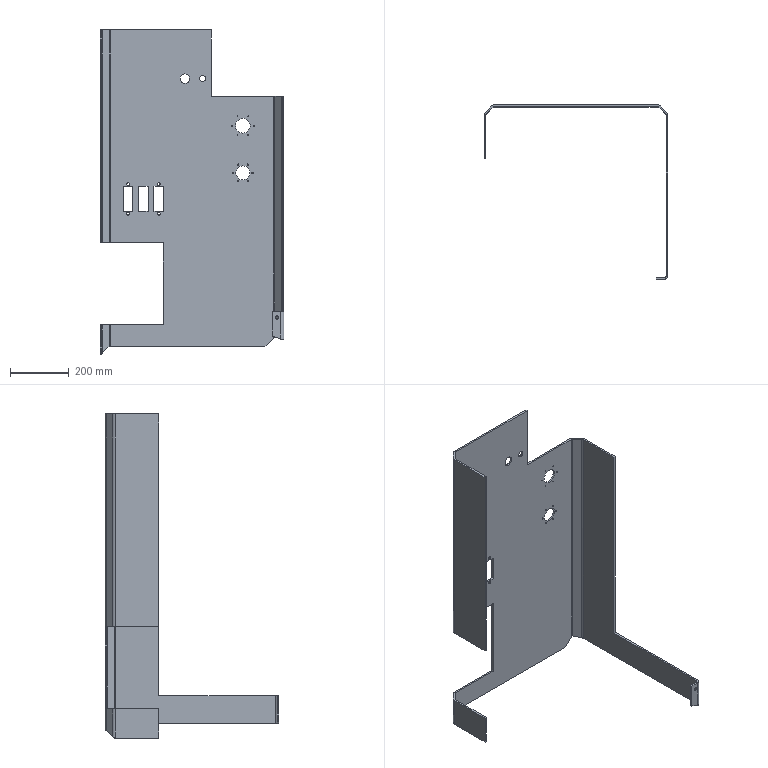Part | SolidWorks | features ICE 8, HoleWzd 2, Fillet 1, FlatPattern 1, SMBaseFlange 1, SheetMetal 1 | 1 solid | 132 faces | box 624 x 590 x 1100 mm | volume 5059916 mm3 | plane 67 | cylinder 58 | spline 7 | commonest cylinder face diameters 3.3 x12 4.2 x12 10 x8 12 x7 24 x7 4 x2